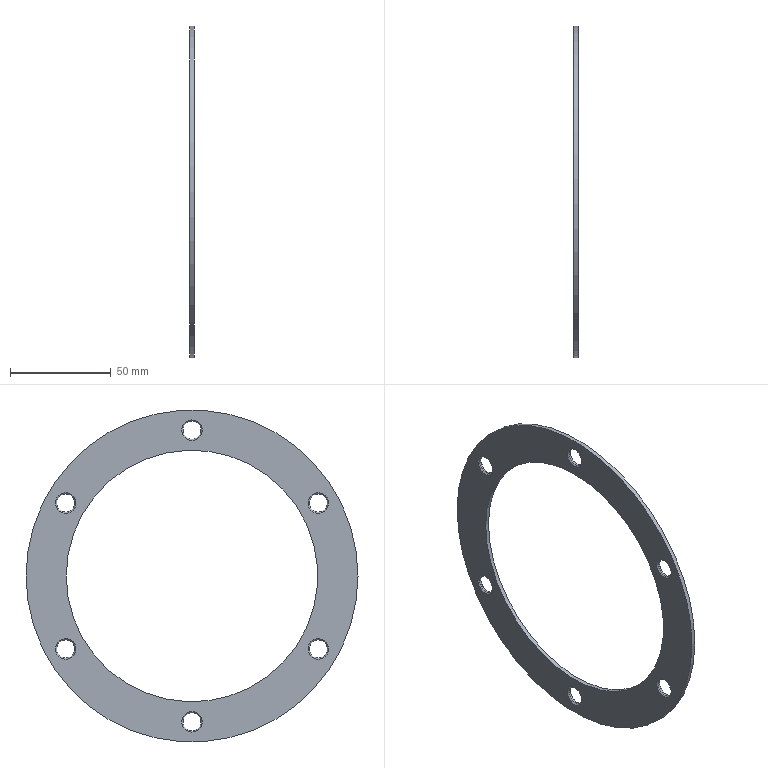Part | NX | 1 solid | 22 faces | box 2 x 165 x 165 mm | volume 17394 mm3 | cone 12 | cylinder 8 | plane 2 | commonest cylinder face diameters 9 x6 125 x1 165 x1
STEP:
#1=CARTESIAN_POINT('',(0.6,-58.89,34.));
#2=VERTEX_POINT('',#1);
#3=CARTESIAN_POINT('',(0.6,-62.787,36.25));
#4=DIRECTION('',(-1.,0.,0.));
#5=DIRECTION('',(0.,0.866,-0.5));
#6=AXIS2_PLACEMENT_3D('',#3,#4,#5);
#7=CIRCLE('',#6,4.5);
#8=EDGE_CURVE('',#2,#2,#7,.T.);
#9=ORIENTED_EDGE('',*,*,#8,.F.);
#10=EDGE_LOOP('',(#9));
#11=FACE_BOUND('',#10,.T.);
#12=CARTESIAN_POINT('',(0.,-58.37,33.7));
#13=VERTEX_POINT('',#12);
#14=CARTESIAN_POINT('',(0.,-62.787,36.25));
#15=DIRECTION('',(1.,0.,0.));
#16=DIRECTION('',(0.,0.866,-0.5));
#17=AXIS2_PLACEMENT_3D('',#14,#15,#16);
#18=CIRCLE('',#17,5.1);
#19=EDGE_CURVE('',#13,#13,#18,.T.);
#20=ORIENTED_EDGE('',*,*,#19,.F.);
#21=EDGE_LOOP('',(#20));
#22=FACE_BOUND('',#21,.T.);
#23=CARTESIAN_POINT('',(0.,-62.787,36.25));
#24=DIRECTION('',(-1.,0.,0.));
#25=DIRECTION('',(0.,0.866,-0.5));
#26=AXIS2_PLACEMENT_3D('',#23,#24,#25);
#27=CONICAL_SURFACE('',#26,5.1,45.);
#28=ADVANCED_FACE('',(#11,#22),#27,.F.);
#29=CARTESIAN_POINT('',(1.4,-58.89,34.));
#30=VERTEX_POINT('',#29);
#31=CARTESIAN_POINT('',(1.4,-62.787,36.25));
#32=DIRECTION('',(1.,0.,0.));
#33=DIRECTION('',(0.,0.866,-0.5));
#34=AXIS2_PLACEMENT_3D('',#31,#32,#33);
#35=CIRCLE('',#34,4.5);
#36=EDGE_CURVE('',#30,#30,#35,.T.);
#37=ORIENTED_EDGE('',*,*,#36,.T.);
#38=EDGE_LOOP('',(#37));
#39=FACE_BOUND('',#38,.T.);
#40=ORIENTED_EDGE('',*,*,#8,.T.);
#41=EDGE_LOOP('',(#40));
#42=FACE_BOUND('',#41,.T.);
#43=CARTESIAN_POINT('',(0.,-62.787,36.25));
#44=DIRECTION('',(1.,0.,0.));
#45=DIRECTION('',(0.,-0.866,0.5));
#46=AXIS2_PLACEMENT_3D('',#43,#44,#45);
#47=CYLINDRICAL_SURFACE('',#46,4.5);
#48=ADVANCED_FACE('',(#39,#42),#47,.F.);
#49=CARTESIAN_POINT('',(2.,-58.37,33.7));
#50=VERTEX_POINT('',#49);
#51=CARTESIAN_POINT('',(2.,-62.787,36.25));
#52=DIRECTION('',(-1.,0.,0.));
#53=DIRECTION('',(0.,0.866,-0.5));
#54=AXIS2_PLACEMENT_3D('',#51,#52,#53);
#55=CIRCLE('',#54,5.1);
#56=EDGE_CURVE('',#50,#50,#55,.T.);
#57=ORIENTED_EDGE('',*,*,#56,.F.);
#58=EDGE_LOOP('',(#57));
#59=FACE_BOUND('',#58,.T.);
#60=ORIENTED_EDGE('',*,*,#36,.F.);
#61=EDGE_LOOP('',(#60));
#62=FACE_BOUND('',#61,.T.);
#63=CARTESIAN_POINT('',(1.4,-62.787,36.25));
#64=DIRECTION('',(1.,0.,0.));
#65=DIRECTION('',(0.,-0.866,0.5));
#66=AXIS2_PLACEMENT_3D('',#63,#64,#65);
#67=CONICAL_SURFACE('',#66,4.5,45.);
#68=ADVANCED_FACE('',(#59,#62),#67,.F.);
#69=CARTESIAN_POINT('',(0.6,-58.89,-34.));
#70=VERTEX_POINT('',#69);
#71=CARTESIAN_POINT('',(0.6,-62.787,-36.25));
#72=DIRECTION('',(-1.,0.,0.));
#73=DIRECTION('',(0.,0.866,0.5));
#74=AXIS2_PLACEMENT_3D('',#71,#72,#73);
#75=CIRCLE('',#74,4.5);
#76=EDGE_CURVE('',#70,#70,#75,.T.);
#77=ORIENTED_EDGE('',*,*,#76,.F.);
#78=EDGE_LOOP('',(#77));
#79=FACE_BOUND('',#78,.T.);
#80=CARTESIAN_POINT('',(0.,-58.37,-33.7));
#81=VERTEX_POINT('',#80);
#82=CARTESIAN_POINT('',(0.,-62.787,-36.25));
#83=DIRECTION('',(1.,0.,0.));
#84=DIRECTION('',(0.,0.866,0.5));
#85=AXIS2_PLACEMENT_3D('',#82,#83,#84);
#86=CIRCLE('',#85,5.1);
#87=EDGE_CURVE('',#81,#81,#86,.T.);
#88=ORIENTED_EDGE('',*,*,#87,.F.);
#89=EDGE_LOOP('',(#88));
#90=FACE_BOUND('',#89,.T.);
#91=CARTESIAN_POINT('',(0.,-62.787,-36.25));
#92=DIRECTION('',(-1.,0.,0.));
#93=DIRECTION('',(0.,0.866,0.5));
#94=AXIS2_PLACEMENT_3D('',#91,#92,#93);
#95=CONICAL_SURFACE('',#94,5.1,45.);
#96=ADVANCED_FACE('',(#79,#90),#95,.F.);
#97=CARTESIAN_POINT('',(1.4,-58.89,-34.));
#98=VERTEX_POINT('',#97);
#99=CARTESIAN_POINT('',(1.4,-62.787,-36.25));
#100=DIRECTION('',(1.,0.,0.));
#101=DIRECTION('',(0.,0.866,0.5));
#102=AXIS2_PLACEMENT_3D('',#99,#100,#101);
#103=CIRCLE('',#102,4.5);
#104=EDGE_CURVE('',#98,#98,#103,.T.);
#105=ORIENTED_EDGE('',*,*,#104,.T.);
#106=EDGE_LOOP('',(#105));
#107=FACE_BOUND('',#106,.T.);
#108=ORIENTED_EDGE('',*,*,#76,.T.);
#109=EDGE_LOOP('',(#108));
#110=FACE_BOUND('',#109,.T.);
#111=CARTESIAN_POINT('',(0.,-62.787,-36.25));
#112=DIRECTION('',(1.,0.,0.));
#113=DIRECTION('',(0.,-0.866,-0.5));
#114=AXIS2_PLACEMENT_3D('',#111,#112,#113);
#115=CYLINDRICAL_SURFACE('',#114,4.5);
#116=ADVANCED_FACE('',(#107,#110),#115,.F.);
#117=CARTESIAN_POINT('',(2.,-58.37,-33.7));
#118=VERTEX_POINT('',#117);
#119=CARTESIAN_POINT('',(2.,-62.787,-36.25));
#120=DIRECTION('',(-1.,0.,0.));
#121=DIRECTION('',(0.,0.866,0.5));
#122=AXIS2_PLACEMENT_3D('',#119,#120,#121);
#123=CIRCLE('',#122,5.1);
#124=EDGE_CURVE('',#118,#118,#123,.T.);
#125=ORIENTED_EDGE('',*,*,#124,.F.);
#126=EDGE_LOOP('',(#125));
#127=FACE_BOUND('',#126,.T.);
#128=ORIENTED_EDGE('',*,*,#104,.F.);
#129=EDGE_LOOP('',(#128));
#130=FACE_BOUND('',#129,.T.);
#131=CARTESIAN_POINT('',(1.4,-62.787,-36.25));
#132=DIRECTION('',(1.,0.,0.));
#133=DIRECTION('',(0.,-0.866,-0.5));
#134=AXIS2_PLACEMENT_3D('',#131,#132,#133);
#135=CONICAL_SURFACE('',#134,4.5,45.);
#136=ADVANCED_FACE('',(#127,#130),#135,.F.);
#137=CARTESIAN_POINT('',(0.6,0.,-68.));
#138=VERTEX_POINT('',#137);
#139=CARTESIAN_POINT('',(0.6,0.,-72.5));
#140=DIRECTION('',(-1.,0.,0.));
#141=DIRECTION('',(0.,0.,1.));
#142=AXIS2_PLACEMENT_3D('',#139,#140,#141);
#143=CIRCLE('',#142,4.5);
#144=EDGE_CURVE('',#138,#138,#143,.T.);
#145=ORIENTED_EDGE('',*,*,#144,.F.);
#146=EDGE_LOOP('',(#145));
#147=FACE_BOUND('',#146,.T.);
#148=CARTESIAN_POINT('',(0.,0.,-67.4));
#149=VERTEX_POINT('',#148);
#150=CARTESIAN_POINT('',(0.,0.,-72.5));
#151=DIRECTION('',(1.,0.,0.));
#152=DIRECTION('',(0.,0.,1.));
#153=AXIS2_PLACEMENT_3D('',#150,#151,#152);
#154=CIRCLE('',#153,5.1);
#155=EDGE_CURVE('',#149,#149,#154,.T.);
#156=ORIENTED_EDGE('',*,*,#155,.F.);
#157=EDGE_LOOP('',(#156));
#158=FACE_BOUND('',#157,.T.);
#159=CARTESIAN_POINT('',(0.,0.,-72.5));
#160=DIRECTION('',(-1.,0.,0.));
#161=DIRECTION('',(0.,0.,1.));
#162=AXIS2_PLACEMENT_3D('',#159,#160,#161);
#163=CONICAL_SURFACE('',#162,5.1,45.);
#164=ADVANCED_FACE('',(#147,#158),#163,.F.);
#165=CARTESIAN_POINT('',(1.4,0.,-68.));
#166=VERTEX_POINT('',#165);
#167=CARTESIAN_POINT('',(1.4,0.,-72.5));
#168=DIRECTION('',(1.,0.,0.));
#169=DIRECTION('',(0.,0.,1.));
#170=AXIS2_PLACEMENT_3D('',#167,#168,#169);
#171=CIRCLE('',#170,4.5);
#172=EDGE_CURVE('',#166,#166,#171,.T.);
#173=ORIENTED_EDGE('',*,*,#172,.T.);
#174=EDGE_LOOP('',(#173));
#175=FACE_BOUND('',#174,.T.);
#176=ORIENTED_EDGE('',*,*,#144,.T.);
#177=EDGE_LOOP('',(#176));
#178=FACE_BOUND('',#177,.T.);
#179=CARTESIAN_POINT('',(0.,0.,-72.5));
#180=DIRECTION('',(1.,0.,0.));
#181=DIRECTION('',(0.,0.,-1.));
#182=AXIS2_PLACEMENT_3D('',#179,#180,#181);
#183=CYLINDRICAL_SURFACE('',#182,4.5);
#184=ADVANCED_FACE('',(#175,#178),#183,.F.);
#185=CARTESIAN_POINT('',(2.,0.,-67.4));
#186=VERTEX_POINT('',#185);
#187=CARTESIAN_POINT('',(2.,0.,-72.5));
#188=DIRECTION('',(-1.,0.,0.));
#189=DIRECTION('',(0.,0.,1.));
#190=AXIS2_PLACEMENT_3D('',#187,#188,#189);
#191=CIRCLE('',#190,5.1);
#192=EDGE_CURVE('',#186,#186,#191,.T.);
#193=ORIENTED_EDGE('',*,*,#192,.F.);
#194=EDGE_LOOP('',(#193));
#195=FACE_BOUND('',#194,.T.);
#196=ORIENTED_EDGE('',*,*,#172,.F.);
#197=EDGE_LOOP('',(#196));
#198=FACE_BOUND('',#197,.T.);
#199=CARTESIAN_POINT('',(1.4,0.,-72.5));
#200=DIRECTION('',(1.,0.,0.));
#201=DIRECTION('',(0.,0.,-1.));
#202=AXIS2_PLACEMENT_3D('',#199,#200,#201);
#203=CONICAL_SURFACE('',#202,4.5,45.);
#204=ADVANCED_FACE('',(#195,#198),#203,.F.);
#205=CARTESIAN_POINT('',(0.6,58.89,-34.));
#206=VERTEX_POINT('',#205);
#207=CARTESIAN_POINT('',(0.6,62.787,-36.25));
#208=DIRECTION('',(-1.,0.,0.));
#209=DIRECTION('',(0.,-0.866,0.5));
#210=AXIS2_PLACEMENT_3D('',#207,#208,#209);
#211=CIRCLE('',#210,4.5);
#212=EDGE_CURVE('',#206,#206,#211,.T.);
#213=ORIENTED_EDGE('',*,*,#212,.F.);
#214=EDGE_LOOP('',(#213));
#215=FACE_BOUND('',#214,.T.);
#216=CARTESIAN_POINT('',(0.,58.37,-33.7));
#217=VERTEX_POINT('',#216);
#218=CARTESIAN_POINT('',(0.,62.787,-36.25));
#219=DIRECTION('',(1.,0.,0.));
#220=DIRECTION('',(0.,-0.866,0.5));
#221=AXIS2_PLACEMENT_3D('',#218,#219,#220);
#222=CIRCLE('',#221,5.1);
#223=EDGE_CURVE('',#217,#217,#222,.T.);
#224=ORIENTED_EDGE('',*,*,#223,.F.);
#225=EDGE_LOOP('',(#224));
#226=FACE_BOUND('',#225,.T.);
#227=CARTESIAN_POINT('',(0.,62.787,-36.25));
#228=DIRECTION('',(-1.,0.,0.));
#229=DIRECTION('',(0.,-0.866,0.5));
#230=AXIS2_PLACEMENT_3D('',#227,#228,#229);
#231=CONICAL_SURFACE('',#230,5.1,45.);
#232=ADVANCED_FACE('',(#215,#226),#231,.F.);
#233=CARTESIAN_POINT('',(1.4,58.89,-34.));
#234=VERTEX_POINT('',#233);
#235=CARTESIAN_POINT('',(1.4,62.787,-36.25));
#236=DIRECTION('',(1.,0.,0.));
#237=DIRECTION('',(0.,-0.866,0.5));
#238=AXIS2_PLACEMENT_3D('',#235,#236,#237);
#239=CIRCLE('',#238,4.5);
#240=EDGE_CURVE('',#234,#234,#239,.T.);
#241=ORIENTED_EDGE('',*,*,#240,.T.);
#242=EDGE_LOOP('',(#241));
#243=FACE_BOUND('',#242,.T.);
#244=ORIENTED_EDGE('',*,*,#212,.T.);
#245=EDGE_LOOP('',(#244));
#246=FACE_BOUND('',#245,.T.);
#247=CARTESIAN_POINT('',(0.,62.787,-36.25));
#248=DIRECTION('',(1.,0.,0.));
#249=DIRECTION('',(0.,0.866,-0.5));
#250=AXIS2_PLACEMENT_3D('',#247,#248,#249);
#251=CYLINDRICAL_SURFACE('',#250,4.5);
#252=ADVANCED_FACE('',(#243,#246),#251,.F.);
#253=CARTESIAN_POINT('',(2.,58.37,-33.7));
#254=VERTEX_POINT('',#253);
#255=CARTESIAN_POINT('',(2.,62.787,-36.25));
#256=DIRECTION('',(-1.,0.,0.));
#257=DIRECTION('',(0.,-0.866,0.5));
#258=AXIS2_PLACEMENT_3D('',#255,#256,#257);
#259=CIRCLE('',#258,5.1);
#260=EDGE_CURVE('',#254,#254,#259,.T.);
#261=ORIENTED_EDGE('',*,*,#260,.F.);
#262=EDGE_LOOP('',(#261));
#263=FACE_BOUND('',#262,.T.);
#264=ORIENTED_EDGE('',*,*,#240,.F.);
#265=EDGE_LOOP('',(#264));
#266=FACE_BOUND('',#265,.T.);
#267=CARTESIAN_POINT('',(1.4,62.787,-36.25));
#268=DIRECTION('',(1.,0.,0.));
#269=DIRECTION('',(0.,0.866,-0.5));
#270=AXIS2_PLACEMENT_3D('',#267,#268,#269);
#271=CONICAL_SURFACE('',#270,4.5,45.);
#272=ADVANCED_FACE('',(#263,#266),#271,.F.);
#273=CARTESIAN_POINT('',(0.6,58.89,34.));
#274=VERTEX_POINT('',#273);
#275=CARTESIAN_POINT('',(0.6,62.787,36.25));
#276=DIRECTION('',(-1.,0.,0.));
#277=DIRECTION('',(0.,-0.866,-0.5));
#278=AXIS2_PLACEMENT_3D('',#275,#276,#277);
#279=CIRCLE('',#278,4.5);
#280=EDGE_CURVE('',#274,#274,#279,.T.);
#281=ORIENTED_EDGE('',*,*,#280,.F.);
#282=EDGE_LOOP('',(#281));
#283=FACE_BOUND('',#282,.T.);
#284=CARTESIAN_POINT('',(0.,58.37,33.7));
#285=VERTEX_POINT('',#284);
#286=CARTESIAN_POINT('',(0.,62.787,36.25));
#287=DIRECTION('',(1.,0.,0.));
#288=DIRECTION('',(0.,-0.866,-0.5));
#289=AXIS2_PLACEMENT_3D('',#286,#287,#288);
#290=CIRCLE('',#289,5.1);
#291=EDGE_CURVE('',#285,#285,#290,.T.);
#292=ORIENTED_EDGE('',*,*,#291,.F.);
#293=EDGE_LOOP('',(#292));
#294=FACE_BOUND('',#293,.T.);
#295=CARTESIAN_POINT('',(0.,62.787,36.25));
#296=DIRECTION('',(-1.,0.,0.));
#297=DIRECTION('',(0.,-0.866,-0.5));
#298=AXIS2_PLACEMENT_3D('',#295,#296,#297);
#299=CONICAL_SURFACE('',#298,5.1,45.);
#300=ADVANCED_FACE('',(#283,#294),#299,.F.);
#301=CARTESIAN_POINT('',(1.4,58.89,34.));
#302=VERTEX_POINT('',#301);
#303=CARTESIAN_POINT('',(1.4,62.787,36.25));
#304=DIRECTION('',(1.,0.,0.));
#305=DIRECTION('',(0.,-0.866,-0.5));
#306=AXIS2_PLACEMENT_3D('',#303,#304,#305);
#307=CIRCLE('',#306,4.5);
#308=EDGE_CURVE('',#302,#302,#307,.T.);
#309=ORIENTED_EDGE('',*,*,#308,.T.);
#310=EDGE_LOOP('',(#309));
#311=FACE_BOUND('',#310,.T.);
#312=ORIENTED_EDGE('',*,*,#280,.T.);
#313=EDGE_LOOP('',(#312));
#314=FACE_BOUND('',#313,.T.);
#315=CARTESIAN_POINT('',(0.,62.787,36.25));
#316=DIRECTION('',(1.,0.,0.));
#317=DIRECTION('',(0.,0.866,0.5));
#318=AXIS2_PLACEMENT_3D('',#315,#316,#317);
#319=CYLINDRICAL_SURFACE('',#318,4.5);
#320=ADVANCED_FACE('',(#311,#314),#319,.F.);
#321=CARTESIAN_POINT('',(2.,58.37,33.7));
#322=VERTEX_POINT('',#321);
#323=CARTESIAN_POINT('',(2.,62.787,36.25));
#324=DIRECTION('',(-1.,0.,0.));
#325=DIRECTION('',(0.,-0.866,-0.5));
#326=AXIS2_PLACEMENT_3D('',#323,#324,#325);
#327=CIRCLE('',#326,5.1);
#328=EDGE_CURVE('',#322,#322,#327,.T.);
#329=ORIENTED_EDGE('',*,*,#328,.F.);
#330=EDGE_LOOP('',(#329));
#331=FACE_BOUND('',#330,.T.);
#332=ORIENTED_EDGE('',*,*,#308,.F.);
#333=EDGE_LOOP('',(#332));
#334=FACE_BOUND('',#333,.T.);
#335=CARTESIAN_POINT('',(1.4,62.787,36.25));
#336=DIRECTION('',(1.,0.,0.));
#337=DIRECTION('',(0.,0.866,0.5));
#338=AXIS2_PLACEMENT_3D('',#335,#336,#337);
#339=CONICAL_SURFACE('',#338,4.5,45.);
#340=ADVANCED_FACE('',(#331,#334),#339,.F.);
#341=CARTESIAN_POINT('',(2.,82.5,0.));
#342=VERTEX_POINT('',#341);
#343=CARTESIAN_POINT('',(2.,0.,0.));
#344=DIRECTION('',(1.,0.,0.));
#345=DIRECTION('',(0.,1.,0.));
#346=AXIS2_PLACEMENT_3D('',#343,#344,#345);
#347=CIRCLE('',#346,82.5);
#348=EDGE_CURVE('',#342,#342,#347,.T.);
#349=ORIENTED_EDGE('',*,*,#348,.F.);
#350=EDGE_LOOP('',(#349));
#351=FACE_BOUND('',#350,.T.);
#352=CARTESIAN_POINT('',(0.,82.5,0.));
#353=VERTEX_POINT('',#352);
#354=CARTESIAN_POINT('',(0.,0.,0.));
#355=DIRECTION('',(1.,0.,0.));
#356=DIRECTION('',(0.,1.,0.));
#357=AXIS2_PLACEMENT_3D('',#354,#355,#356);
#358=CIRCLE('',#357,82.5);
#359=EDGE_CURVE('',#353,#353,#358,.T.);
#360=ORIENTED_EDGE('',*,*,#359,.T.);
#361=EDGE_LOOP('',(#360));
#362=FACE_BOUND('',#361,.T.);
#363=CARTESIAN_POINT('',(2.,0.,0.));
#364=DIRECTION('',(-1.,0.,0.));
#365=DIRECTION('',(0.,0.,-1.));
#366=AXIS2_PLACEMENT_3D('',#363,#364,#365);
#367=CYLINDRICAL_SURFACE('',#366,82.5);
#368=ADVANCED_FACE('',(#351,#362),#367,.T.);
#369=CARTESIAN_POINT('',(2.,62.5,0.));
#370=VERTEX_POINT('',#369);
#371=CARTESIAN_POINT('',(2.,0.,0.));
#372=DIRECTION('',(1.,0.,0.));
#373=DIRECTION('',(0.,1.,0.));
#374=AXIS2_PLACEMENT_3D('',#371,#372,#373);
#375=CIRCLE('',#374,62.5);
#376=EDGE_CURVE('',#370,#370,#375,.T.);
#377=ORIENTED_EDGE('',*,*,#376,.T.);
#378=EDGE_LOOP('',(#377));
#379=FACE_BOUND('',#378,.T.);
#380=CARTESIAN_POINT('',(0.,62.5,0.));
#381=VERTEX_POINT('',#380);
#382=CARTESIAN_POINT('',(0.,0.,0.));
#383=DIRECTION('',(1.,0.,0.));
#384=DIRECTION('',(0.,1.,0.));
#385=AXIS2_PLACEMENT_3D('',#382,#383,#384);
#386=CIRCLE('',#385,62.5);
#387=EDGE_CURVE('',#381,#381,#386,.T.);
#388=ORIENTED_EDGE('',*,*,#387,.F.);
#389=EDGE_LOOP('',(#388));
#390=FACE_BOUND('',#389,.T.);
#391=CARTESIAN_POINT('',(2.,0.,0.));
#392=DIRECTION('',(-1.,0.,0.));
#393=DIRECTION('',(0.,0.,-1.));
#394=AXIS2_PLACEMENT_3D('',#391,#392,#393);
#395=CYLINDRICAL_SURFACE('',#394,62.5);
#396=ADVANCED_FACE('',(#379,#390),#395,.F.);
#397=ORIENTED_EDGE('',*,*,#56,.T.);
#398=EDGE_LOOP('',(#397));
#399=FACE_BOUND('',#398,.T.);
#400=ORIENTED_EDGE('',*,*,#124,.T.);
#401=EDGE_LOOP('',(#400));
#402=FACE_BOUND('',#401,.T.);
#403=ORIENTED_EDGE('',*,*,#192,.T.);
#404=EDGE_LOOP('',(#403));
#405=FACE_BOUND('',#404,.T.);
#406=ORIENTED_EDGE('',*,*,#260,.T.);
#407=EDGE_LOOP('',(#406));
#408=FACE_BOUND('',#407,.T.);
#409=ORIENTED_EDGE('',*,*,#328,.T.);
#410=EDGE_LOOP('',(#409));
#411=FACE_BOUND('',#410,.T.);
#412=CARTESIAN_POINT('',(2.,0.,67.4));
#413=VERTEX_POINT('',#412);
#414=CARTESIAN_POINT('',(2.,0.,72.5));
#415=DIRECTION('',(-1.,0.,0.));
#416=DIRECTION('',(0.,0.,-1.));
#417=AXIS2_PLACEMENT_3D('',#414,#415,#416);
#418=CIRCLE('',#417,5.1);
#419=EDGE_CURVE('',#413,#413,#418,.T.);
#420=ORIENTED_EDGE('',*,*,#419,.T.);
#421=EDGE_LOOP('',(#420));
#422=FACE_BOUND('',#421,.T.);
#423=ORIENTED_EDGE('',*,*,#348,.T.);
#424=EDGE_LOOP('',(#423));
#425=FACE_BOUND('',#424,.T.);
#426=ORIENTED_EDGE('',*,*,#376,.F.);
#427=EDGE_LOOP('',(#426));
#428=FACE_BOUND('',#427,.T.);
#429=CARTESIAN_POINT('',(2.,0.,0.));
#430=DIRECTION('',(1.,0.,0.));
#431=DIRECTION('',(0.,0.,1.));
#432=AXIS2_PLACEMENT_3D('',#429,#430,#431);
#433=PLANE('',#432);
#434=ADVANCED_FACE('',(#399,#402,#405,#408,#411,#422,#425,#428),#433,.T.);
#435=ORIENTED_EDGE('',*,*,#19,.T.);
#436=EDGE_LOOP('',(#435));
#437=FACE_BOUND('',#436,.T.);
#438=ORIENTED_EDGE('',*,*,#87,.T.);
#439=EDGE_LOOP('',(#438));
#440=FACE_BOUND('',#439,.T.);
#441=ORIENTED_EDGE('',*,*,#155,.T.);
#442=EDGE_LOOP('',(#441));
#443=FACE_BOUND('',#442,.T.);
#444=ORIENTED_EDGE('',*,*,#223,.T.);
#445=EDGE_LOOP('',(#444));
#446=FACE_BOUND('',#445,.T.);
#447=ORIENTED_EDGE('',*,*,#291,.T.);
#448=EDGE_LOOP('',(#447));
#449=FACE_BOUND('',#448,.T.);
#450=CARTESIAN_POINT('',(0.,0.,67.4));
#451=VERTEX_POINT('',#450);
#452=CARTESIAN_POINT('',(0.,0.,72.5));
#453=DIRECTION('',(1.,0.,0.));
#454=DIRECTION('',(0.,0.,-1.));
#455=AXIS2_PLACEMENT_3D('',#452,#453,#454);
#456=CIRCLE('',#455,5.1);
#457=EDGE_CURVE('',#451,#451,#456,.T.);
#458=ORIENTED_EDGE('',*,*,#457,.T.);
#459=EDGE_LOOP('',(#458));
#460=FACE_BOUND('',#459,.T.);
#461=ORIENTED_EDGE('',*,*,#359,.F.);
#462=EDGE_LOOP('',(#461));
#463=FACE_BOUND('',#462,.T.);
#464=ORIENTED_EDGE('',*,*,#387,.T.);
#465=EDGE_LOOP('',(#464));
#466=FACE_BOUND('',#465,.T.);
#467=CARTESIAN_POINT('',(0.,0.,0.));
#468=DIRECTION('',(1.,0.,0.));
#469=DIRECTION('',(0.,0.,1.));
#470=AXIS2_PLACEMENT_3D('',#467,#468,#469);
#471=PLANE('',#470);
#472=ADVANCED_FACE('',(#437,#440,#443,#446,#449,#460,#463,#466),#471,.F.);
#473=CARTESIAN_POINT('',(1.4,0.,68.));
#474=VERTEX_POINT('',#473);
#475=CARTESIAN_POINT('',(1.4,0.,72.5));
#476=DIRECTION('',(1.,0.,0.));
#477=DIRECTION('',(0.,0.,-1.));
#478=AXIS2_PLACEMENT_3D('',#475,#476,#477);
#479=CIRCLE('',#478,4.5);
#480=EDGE_CURVE('',#474,#474,#479,.T.);
#481=ORIENTED_EDGE('',*,*,#480,.T.);
#482=EDGE_LOOP('',(#481));
#483=FACE_BOUND('',#482,.T.);
#484=CARTESIAN_POINT('',(0.6,0.,68.));
#485=VERTEX_POINT('',#484);
#486=CARTESIAN_POINT('',(0.6,0.,72.5));
#487=DIRECTION('',(-1.,0.,0.));
#488=DIRECTION('',(0.,0.,-1.));
#489=AXIS2_PLACEMENT_3D('',#486,#487,#488);
#490=CIRCLE('',#489,4.5);
#491=EDGE_CURVE('',#485,#485,#490,.T.);
#492=ORIENTED_EDGE('',*,*,#491,.T.);
#493=EDGE_LOOP('',(#492));
#494=FACE_BOUND('',#493,.T.);
#495=CARTESIAN_POINT('',(0.,0.,72.5));
#496=DIRECTION('',(1.,0.,0.));
#497=DIRECTION('',(0.,0.,1.));
#498=AXIS2_PLACEMENT_3D('',#495,#496,#497);
#499=CYLINDRICAL_SURFACE('',#498,4.5);
#500=ADVANCED_FACE('',(#483,#494),#499,.F.);
#501=ORIENTED_EDGE('',*,*,#491,.F.);
#502=EDGE_LOOP('',(#501));
#503=FACE_BOUND('',#502,.T.);
#504=ORIENTED_EDGE('',*,*,#457,.F.);
#505=EDGE_LOOP('',(#504));
#506=FACE_BOUND('',#505,.T.);
#507=CARTESIAN_POINT('',(0.,0.,72.5));
#508=DIRECTION('',(-1.,0.,0.));
#509=DIRECTION('',(0.,0.,-1.));
#510=AXIS2_PLACEMENT_3D('',#507,#508,#509);
#511=CONICAL_SURFACE('',#510,5.1,45.);
#512=ADVANCED_FACE('',(#503,#506),#511,.F.);
#513=ORIENTED_EDGE('',*,*,#419,.F.);
#514=EDGE_LOOP('',(#513));
#515=FACE_BOUND('',#514,.T.);
#516=ORIENTED_EDGE('',*,*,#480,.F.);
#517=EDGE_LOOP('',(#516));
#518=FACE_BOUND('',#517,.T.);
#519=CARTESIAN_POINT('',(1.4,0.,72.5));
#520=DIRECTION('',(1.,0.,0.));
#521=DIRECTION('',(0.,0.,1.));
#522=AXIS2_PLACEMENT_3D('',#519,#520,#521);
#523=CONICAL_SURFACE('',#522,4.5,45.);
#524=ADVANCED_FACE('',(#515,#518),#523,.F.);
#525=CLOSED_SHELL('',(#28,#48,#68,#96,#116,#136,#164,#184,#204,#232,#252,#272,#300,#320,#340,#368,#396,#434,#472,#500,#512,#524));
#526=MANIFOLD_SOLID_BREP('',#525);
#527=(LENGTH_UNIT()NAMED_UNIT(*)SI_UNIT(.MILLI.,.METRE.));
#528=UNCERTAINTY_MEASURE_WITH_UNIT(LENGTH_MEASURE(0.00002),#527,'','');
#529=(NAMED_UNIT(*)PLANE_ANGLE_UNIT()SI_UNIT($,.RADIAN.));
#530=PLANE_ANGLE_MEASURE_WITH_UNIT(PLANE_ANGLE_MEASURE(0.01745),#529);
#531=DIMENSIONAL_EXPONENTS(0.,0.,0.,0.,0.,0.,0.);
#532=(CONVERSION_BASED_UNIT('DEGREE',#530)NAMED_UNIT(#531)PLANE_ANGLE_UNIT());
#533=(NAMED_UNIT(*)SI_UNIT($,.STERADIAN.)SOLID_ANGLE_UNIT());
#534=(GEOMETRIC_REPRESENTATION_CONTEXT(3)GLOBAL_UNCERTAINTY_ASSIGNED_CONTEXT((#528))GLOBAL_UNIT_ASSIGNED_CONTEXT((#527,#532,#533))REPRESENTATION_CONTEXT('',''));
#535=ADVANCED_BREP_SHAPE_REPRESENTATION('',(#526),#534);